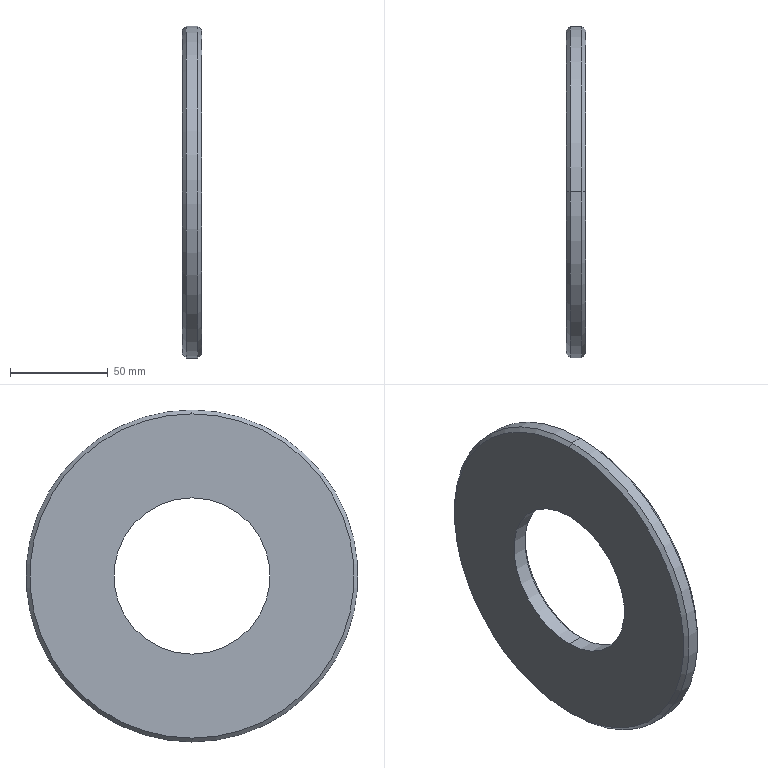Part | SolidWorks | features Chamfer 1, Extrusion 1 | 1 solid | 12 faces | box 10 x 170 x 170 mm | volume 174084 mm3 | cone 6 | cylinder 4 | plane 2 | commonest cylinder face diameters 80 x2 170 x2
STEP:
#1=CARTESIAN_POINT('',(8.,0.,40.));
#2=VERTEX_POINT('',#1);
#3=CARTESIAN_POINT('',(8.,0.,-40.));
#4=VERTEX_POINT('',#3);
#5=CARTESIAN_POINT('',(8.,0.,0.));
#6=DIRECTION('',(1.,0.,0.));
#7=DIRECTION('',(0.,0.,-1.));
#8=AXIS2_PLACEMENT_3D('',#5,#6,#7);
#9=CIRCLE('',#8,40.);
#10=EDGE_CURVE('',#2,#4,#9,.T.);
#11=ORIENTED_EDGE('',*,*,#10,.F.);
#12=CARTESIAN_POINT('',(10.,0.,42.));
#13=VERTEX_POINT('',#12);
#14=CARTESIAN_POINT('',(8.,0.,40.));
#15=DIRECTION('',(0.7071,0.,0.7071));
#16=VECTOR('',#15,1000.);
#17=LINE('',#14,#16);
#18=EDGE_CURVE('',#2,#13,#17,.T.);
#19=ORIENTED_EDGE('',*,*,#18,.T.);
#20=CARTESIAN_POINT('',(10.,0.,-42.));
#21=VERTEX_POINT('',#20);
#22=CARTESIAN_POINT('',(10.,0.,0.));
#23=DIRECTION('',(-1.,0.,0.));
#24=DIRECTION('',(0.,0.,-1.));
#25=AXIS2_PLACEMENT_3D('',#22,#23,#24);
#26=CIRCLE('',#25,42.);
#27=EDGE_CURVE('',#21,#13,#26,.T.);
#28=ORIENTED_EDGE('',*,*,#27,.F.);
#29=CARTESIAN_POINT('',(8.,0.,-40.));
#30=DIRECTION('',(0.7071,0.,-0.7071));
#31=VECTOR('',#30,1000.);
#32=LINE('',#29,#31);
#33=EDGE_CURVE('',#4,#21,#32,.T.);
#34=ORIENTED_EDGE('',*,*,#33,.F.);
#35=EDGE_LOOP('',(#11,#19,#28,#34));
#36=FACE_OUTER_BOUND('',#35,.T.);
#37=CARTESIAN_POINT('',(8.,0.,0.));
#38=DIRECTION('',(1.,0.,0.));
#39=DIRECTION('',(0.,0.,-1.));
#40=AXIS2_PLACEMENT_3D('',#37,#38,#39);
#41=CONICAL_SURFACE('',#40,40.,0.7854);
#42=ADVANCED_FACE('',(#36),#41,.F.);
#43=CARTESIAN_POINT('',(10.,0.,-83.));
#44=VERTEX_POINT('',#43);
#45=CARTESIAN_POINT('',(10.,0.,83.));
#46=VERTEX_POINT('',#45);
#47=CARTESIAN_POINT('',(10.,0.,0.));
#48=DIRECTION('',(1.,0.,0.));
#49=DIRECTION('',(0.,0.,-1.));
#50=AXIS2_PLACEMENT_3D('',#47,#48,#49);
#51=CIRCLE('',#50,83.);
#52=EDGE_CURVE('',#44,#46,#51,.T.);
#53=ORIENTED_EDGE('',*,*,#52,.F.);
#54=CARTESIAN_POINT('',(8.,0.,-85.));
#55=VERTEX_POINT('',#54);
#56=CARTESIAN_POINT('',(10.,0.,-83.));
#57=DIRECTION('',(-0.7071,0.,-0.7071));
#58=VECTOR('',#57,1000.);
#59=LINE('',#56,#58);
#60=EDGE_CURVE('',#44,#55,#59,.T.);
#61=ORIENTED_EDGE('',*,*,#60,.T.);
#62=CARTESIAN_POINT('',(8.,0.,85.));
#63=VERTEX_POINT('',#62);
#64=CARTESIAN_POINT('',(8.,0.,0.));
#65=DIRECTION('',(-1.,0.,0.));
#66=DIRECTION('',(0.,0.,-1.));
#67=AXIS2_PLACEMENT_3D('',#64,#65,#66);
#68=CIRCLE('',#67,85.);
#69=EDGE_CURVE('',#63,#55,#68,.T.);
#70=ORIENTED_EDGE('',*,*,#69,.F.);
#71=CARTESIAN_POINT('',(10.,0.,83.));
#72=DIRECTION('',(-0.7071,0.,0.7071));
#73=VECTOR('',#72,1000.);
#74=LINE('',#71,#73);
#75=EDGE_CURVE('',#46,#63,#74,.T.);
#76=ORIENTED_EDGE('',*,*,#75,.F.);
#77=EDGE_LOOP('',(#53,#61,#70,#76));
#78=FACE_OUTER_BOUND('',#77,.T.);
#79=CARTESIAN_POINT('',(10.,0.,0.));
#80=DIRECTION('',(-1.,0.,0.));
#81=DIRECTION('',(0.,0.,1.));
#82=AXIS2_PLACEMENT_3D('',#79,#80,#81);
#83=CONICAL_SURFACE('',#82,83.,0.7854);
#84=ADVANCED_FACE('',(#78),#83,.T.);
#85=CARTESIAN_POINT('',(0.,0.,83.));
#86=VERTEX_POINT('',#85);
#87=CARTESIAN_POINT('',(0.,0.,-83.));
#88=VERTEX_POINT('',#87);
#89=CARTESIAN_POINT('',(0.,0.,0.));
#90=DIRECTION('',(-1.,0.,0.));
#91=DIRECTION('',(0.,0.,-1.));
#92=AXIS2_PLACEMENT_3D('',#89,#90,#91);
#93=CIRCLE('',#92,83.);
#94=EDGE_CURVE('',#86,#88,#93,.T.);
#95=ORIENTED_EDGE('',*,*,#94,.F.);
#96=CARTESIAN_POINT('',(2.,0.,85.));
#97=VERTEX_POINT('',#96);
#98=CARTESIAN_POINT('',(2.,0.,85.));
#99=DIRECTION('',(0.7071,0.,0.7071));
#100=VECTOR('',#99,1000.);
#101=LINE('',#98,#100);
#102=EDGE_CURVE('',#86,#97,#101,.T.);
#103=ORIENTED_EDGE('',*,*,#102,.T.);
#104=CARTESIAN_POINT('',(2.,0.,-85.));
#105=VERTEX_POINT('',#104);
#106=CARTESIAN_POINT('',(2.,0.,0.));
#107=DIRECTION('',(1.,0.,0.));
#108=DIRECTION('',(0.,0.,-1.));
#109=AXIS2_PLACEMENT_3D('',#106,#107,#108);
#110=CIRCLE('',#109,85.);
#111=EDGE_CURVE('',#105,#97,#110,.T.);
#112=ORIENTED_EDGE('',*,*,#111,.F.);
#113=CARTESIAN_POINT('',(2.,0.,-85.));
#114=DIRECTION('',(0.7071,0.,-0.7071));
#115=VECTOR('',#114,1000.);
#116=LINE('',#113,#115);
#117=EDGE_CURVE('',#88,#105,#116,.T.);
#118=ORIENTED_EDGE('',*,*,#117,.F.);
#119=EDGE_LOOP('',(#95,#103,#112,#118));
#120=FACE_OUTER_BOUND('',#119,.T.);
#121=CARTESIAN_POINT('',(2.,0.,0.));
#122=DIRECTION('',(1.,0.,0.));
#123=DIRECTION('',(0.,0.,-1.));
#124=AXIS2_PLACEMENT_3D('',#121,#122,#123);
#125=CONICAL_SURFACE('',#124,85.,0.7854);
#126=ADVANCED_FACE('',(#120),#125,.T.);
#127=ORIENTED_EDGE('',*,*,#10,.T.);
#128=CARTESIAN_POINT('',(0.,0.,-40.));
#129=VERTEX_POINT('',#128);
#130=CARTESIAN_POINT('',(10.,0.,-40.));
#131=DIRECTION('',(-1.,0.,0.));
#132=VECTOR('',#131,1000.);
#133=LINE('',#130,#132);
#134=EDGE_CURVE('',#4,#129,#133,.T.);
#135=ORIENTED_EDGE('',*,*,#134,.T.);
#136=CARTESIAN_POINT('',(0.,0.,40.));
#137=VERTEX_POINT('',#136);
#138=CARTESIAN_POINT('',(0.,0.,0.));
#139=DIRECTION('',(1.,0.,0.));
#140=DIRECTION('',(0.,0.,-1.));
#141=AXIS2_PLACEMENT_3D('',#138,#139,#140);
#142=CIRCLE('',#141,40.);
#143=EDGE_CURVE('',#137,#129,#142,.T.);
#144=ORIENTED_EDGE('',*,*,#143,.F.);
#145=CARTESIAN_POINT('',(10.,0.,40.));
#146=DIRECTION('',(-1.,0.,0.));
#147=VECTOR('',#146,1000.);
#148=LINE('',#145,#147);
#149=EDGE_CURVE('',#2,#137,#148,.T.);
#150=ORIENTED_EDGE('',*,*,#149,.F.);
#151=EDGE_LOOP('',(#127,#135,#144,#150));
#152=FACE_OUTER_BOUND('',#151,.T.);
#153=CARTESIAN_POINT('',(10.,0.,0.));
#154=DIRECTION('',(-1.,0.,0.));
#155=DIRECTION('',(0.,0.,1.));
#156=AXIS2_PLACEMENT_3D('',#153,#154,#155);
#157=CYLINDRICAL_SURFACE('',#156,40.);
#158=ADVANCED_FACE('',(#152),#157,.F.);
#159=ORIENTED_EDGE('',*,*,#69,.T.);
#160=CARTESIAN_POINT('',(10.,0.,-85.));
#161=DIRECTION('',(-1.,0.,0.));
#162=VECTOR('',#161,1000.);
#163=LINE('',#160,#162);
#164=EDGE_CURVE('',#55,#105,#163,.T.);
#165=ORIENTED_EDGE('',*,*,#164,.T.);
#166=ORIENTED_EDGE('',*,*,#111,.T.);
#167=CARTESIAN_POINT('',(10.,0.,85.));
#168=DIRECTION('',(-1.,0.,0.));
#169=VECTOR('',#168,1000.);
#170=LINE('',#167,#169);
#171=EDGE_CURVE('',#63,#97,#170,.T.);
#172=ORIENTED_EDGE('',*,*,#171,.F.);
#173=EDGE_LOOP('',(#159,#165,#166,#172));
#174=FACE_OUTER_BOUND('',#173,.T.);
#175=CARTESIAN_POINT('',(10.,0.,0.));
#176=DIRECTION('',(-1.,0.,0.));
#177=DIRECTION('',(0.,0.,1.));
#178=AXIS2_PLACEMENT_3D('',#175,#176,#177);
#179=CYLINDRICAL_SURFACE('',#178,85.);
#180=ADVANCED_FACE('',(#174),#179,.T.);
#181=CARTESIAN_POINT('',(10.,0.,0.));
#182=DIRECTION('',(1.,0.,0.));
#183=DIRECTION('',(0.,0.,-1.));
#184=AXIS2_PLACEMENT_3D('',#181,#182,#183);
#185=CIRCLE('',#184,83.);
#186=EDGE_CURVE('',#46,#44,#185,.T.);
#187=ORIENTED_EDGE('',*,*,#186,.T.);
#188=ORIENTED_EDGE('',*,*,#52,.T.);
#189=EDGE_LOOP('',(#187,#188));
#190=FACE_OUTER_BOUND('',#189,.T.);
#191=ORIENTED_EDGE('',*,*,#27,.T.);
#192=CARTESIAN_POINT('',(10.,0.,0.));
#193=DIRECTION('',(-1.,0.,0.));
#194=DIRECTION('',(0.,0.,-1.));
#195=AXIS2_PLACEMENT_3D('',#192,#193,#194);
#196=CIRCLE('',#195,42.);
#197=EDGE_CURVE('',#13,#21,#196,.T.);
#198=ORIENTED_EDGE('',*,*,#197,.T.);
#199=EDGE_LOOP('',(#191,#198));
#200=FACE_BOUND('',#199,.T.);
#201=CARTESIAN_POINT('',(10.,0.,0.));
#202=DIRECTION('',(1.,0.,0.));
#203=DIRECTION('',(0.,0.,-1.));
#204=AXIS2_PLACEMENT_3D('',#201,#202,#203);
#205=PLANE('',#204);
#206=ADVANCED_FACE('',(#190,#200),#205,.T.);
#207=CARTESIAN_POINT('',(0.,0.,0.));
#208=DIRECTION('',(-1.,0.,0.));
#209=DIRECTION('',(0.,0.,-1.));
#210=AXIS2_PLACEMENT_3D('',#207,#208,#209);
#211=CIRCLE('',#210,83.);
#212=EDGE_CURVE('',#88,#86,#211,.T.);
#213=ORIENTED_EDGE('',*,*,#212,.T.);
#214=ORIENTED_EDGE('',*,*,#94,.T.);
#215=EDGE_LOOP('',(#213,#214));
#216=FACE_OUTER_BOUND('',#215,.T.);
#217=ORIENTED_EDGE('',*,*,#143,.T.);
#218=CARTESIAN_POINT('',(0.,0.,0.));
#219=DIRECTION('',(1.,0.,0.));
#220=DIRECTION('',(0.,0.,-1.));
#221=AXIS2_PLACEMENT_3D('',#218,#219,#220);
#222=CIRCLE('',#221,40.);
#223=EDGE_CURVE('',#129,#137,#222,.T.);
#224=ORIENTED_EDGE('',*,*,#223,.T.);
#225=EDGE_LOOP('',(#217,#224));
#226=FACE_BOUND('',#225,.T.);
#227=CARTESIAN_POINT('',(0.,0.,0.));
#228=DIRECTION('',(1.,0.,0.));
#229=DIRECTION('',(0.,0.,-1.));
#230=AXIS2_PLACEMENT_3D('',#227,#228,#229);
#231=PLANE('',#230);
#232=ADVANCED_FACE('',(#216,#226),#231,.F.);
#233=ORIENTED_EDGE('',*,*,#164,.F.);
#234=CARTESIAN_POINT('',(8.,0.,0.));
#235=DIRECTION('',(-1.,0.,0.));
#236=DIRECTION('',(0.,0.,-1.));
#237=AXIS2_PLACEMENT_3D('',#234,#235,#236);
#238=CIRCLE('',#237,85.);
#239=EDGE_CURVE('',#55,#63,#238,.T.);
#240=ORIENTED_EDGE('',*,*,#239,.T.);
#241=ORIENTED_EDGE('',*,*,#171,.T.);
#242=CARTESIAN_POINT('',(2.,0.,0.));
#243=DIRECTION('',(1.,0.,0.));
#244=DIRECTION('',(0.,0.,-1.));
#245=AXIS2_PLACEMENT_3D('',#242,#243,#244);
#246=CIRCLE('',#245,85.);
#247=EDGE_CURVE('',#97,#105,#246,.T.);
#248=ORIENTED_EDGE('',*,*,#247,.T.);
#249=EDGE_LOOP('',(#233,#240,#241,#248));
#250=FACE_OUTER_BOUND('',#249,.T.);
#251=CARTESIAN_POINT('',(10.,0.,0.));
#252=DIRECTION('',(-1.,0.,0.));
#253=DIRECTION('',(0.,0.,1.));
#254=AXIS2_PLACEMENT_3D('',#251,#252,#253);
#255=CYLINDRICAL_SURFACE('',#254,85.);
#256=ADVANCED_FACE('',(#250),#255,.T.);
#257=ORIENTED_EDGE('',*,*,#134,.F.);
#258=CARTESIAN_POINT('',(8.,0.,0.));
#259=DIRECTION('',(1.,0.,0.));
#260=DIRECTION('',(0.,0.,-1.));
#261=AXIS2_PLACEMENT_3D('',#258,#259,#260);
#262=CIRCLE('',#261,40.);
#263=EDGE_CURVE('',#4,#2,#262,.T.);
#264=ORIENTED_EDGE('',*,*,#263,.T.);
#265=ORIENTED_EDGE('',*,*,#149,.T.);
#266=ORIENTED_EDGE('',*,*,#223,.F.);
#267=EDGE_LOOP('',(#257,#264,#265,#266));
#268=FACE_OUTER_BOUND('',#267,.T.);
#269=CARTESIAN_POINT('',(10.,0.,0.));
#270=DIRECTION('',(-1.,0.,0.));
#271=DIRECTION('',(0.,0.,1.));
#272=AXIS2_PLACEMENT_3D('',#269,#270,#271);
#273=CYLINDRICAL_SURFACE('',#272,40.);
#274=ADVANCED_FACE('',(#268),#273,.F.);
#275=ORIENTED_EDGE('',*,*,#102,.F.);
#276=ORIENTED_EDGE('',*,*,#212,.F.);
#277=ORIENTED_EDGE('',*,*,#117,.T.);
#278=ORIENTED_EDGE('',*,*,#247,.F.);
#279=EDGE_LOOP('',(#275,#276,#277,#278));
#280=FACE_OUTER_BOUND('',#279,.T.);
#281=CARTESIAN_POINT('',(2.,0.,0.));
#282=DIRECTION('',(1.,0.,0.));
#283=DIRECTION('',(0.,0.,-1.));
#284=AXIS2_PLACEMENT_3D('',#281,#282,#283);
#285=CONICAL_SURFACE('',#284,85.,0.7854);
#286=ADVANCED_FACE('',(#280),#285,.T.);
#287=ORIENTED_EDGE('',*,*,#60,.F.);
#288=ORIENTED_EDGE('',*,*,#186,.F.);
#289=ORIENTED_EDGE('',*,*,#75,.T.);
#290=ORIENTED_EDGE('',*,*,#239,.F.);
#291=EDGE_LOOP('',(#287,#288,#289,#290));
#292=FACE_OUTER_BOUND('',#291,.T.);
#293=CARTESIAN_POINT('',(10.,0.,0.));
#294=DIRECTION('',(-1.,0.,0.));
#295=DIRECTION('',(0.,0.,1.));
#296=AXIS2_PLACEMENT_3D('',#293,#294,#295);
#297=CONICAL_SURFACE('',#296,83.,0.7854);
#298=ADVANCED_FACE('',(#292),#297,.T.);
#299=ORIENTED_EDGE('',*,*,#18,.F.);
#300=ORIENTED_EDGE('',*,*,#263,.F.);
#301=ORIENTED_EDGE('',*,*,#33,.T.);
#302=ORIENTED_EDGE('',*,*,#197,.F.);
#303=EDGE_LOOP('',(#299,#300,#301,#302));
#304=FACE_OUTER_BOUND('',#303,.T.);
#305=CARTESIAN_POINT('',(8.,0.,0.));
#306=DIRECTION('',(1.,0.,0.));
#307=DIRECTION('',(0.,0.,-1.));
#308=AXIS2_PLACEMENT_3D('',#305,#306,#307);
#309=CONICAL_SURFACE('',#308,40.,0.7854);
#310=ADVANCED_FACE('',(#304),#309,.F.);
#311=CLOSED_SHELL('',(#42,#84,#126,#158,#180,#206,#232,#256,#274,#286,#298,#310));
#312=MANIFOLD_SOLID_BREP('',#311);
#313=CARTESIAN_POINT('',(0.,0.,0.));
#314=DIRECTION('',(0.,0.,1.));
#315=DIRECTION('',(1.,0.,0.));
#316=AXIS2_PLACEMENT_3D('',#313,#314,#315);
#317=(LENGTH_UNIT()NAMED_UNIT(*)SI_UNIT(.MILLI.,.METRE.));
#318=UNCERTAINTY_MEASURE_WITH_UNIT(LENGTH_MEASURE(0.00001),#317,'','');
#319=(NAMED_UNIT(*)PLANE_ANGLE_UNIT()SI_UNIT($,.RADIAN.));
#320=(NAMED_UNIT(*)SI_UNIT($,.STERADIAN.)SOLID_ANGLE_UNIT());
#321=(GEOMETRIC_REPRESENTATION_CONTEXT(3)GLOBAL_UNCERTAINTY_ASSIGNED_CONTEXT((#318))GLOBAL_UNIT_ASSIGNED_CONTEXT((#317,#319,#320))REPRESENTATION_CONTEXT('',''));
#322=ADVANCED_BREP_SHAPE_REPRESENTATION('',(#312,#316),#321);